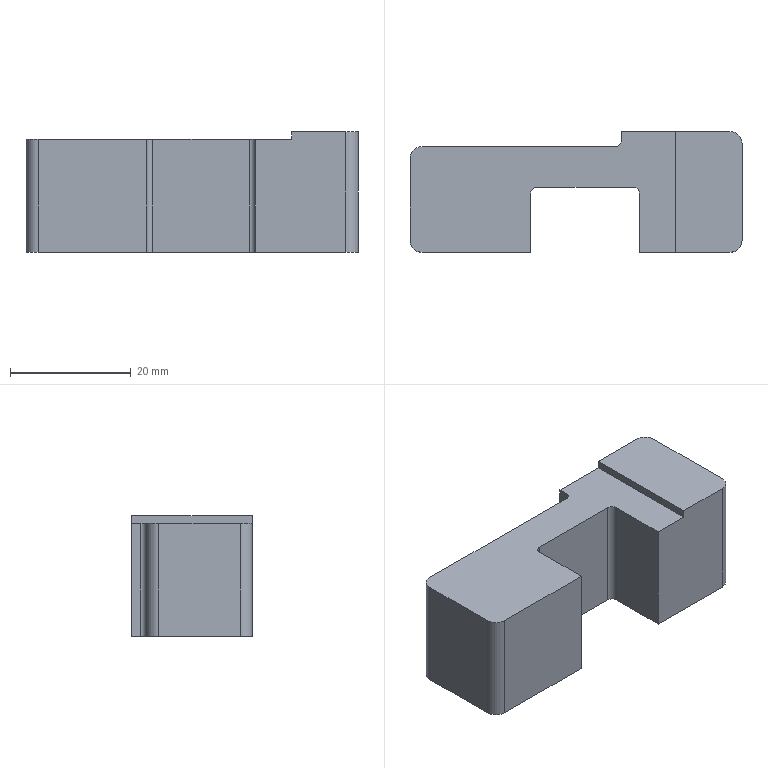Part | STEP file | 03-20 product pre-press block | 1 solid | 29 faces | box 55 x 20 x 20 mm | volume 15350 mm3 | plane 14 | cylinder 11 | cone 4 | commonest cylinder face diameters 3.3 x4 4 x4 2 x3
STEP:
#1=CARTESIAN_POINT('',(21.15,0.,10.1));
#2=VERTEX_POINT('',#1);
#3=CARTESIAN_POINT('',(17.85,0.,10.1));
#4=VERTEX_POINT('',#3);
#5=CARTESIAN_POINT('',(19.5,0.,10.1));
#6=DIRECTION('',(0.,0.,-1.));
#7=DIRECTION('',(-1.,0.,0.));
#8=AXIS2_PLACEMENT_3D('',#5,#6,#7);
#9=CIRCLE('',#8,1.65);
#10=EDGE_CURVE('',#2,#4,#9,.T.);
#11=ORIENTED_EDGE('',*,*,#10,.F.);
#12=CARTESIAN_POINT('',(21.15,0.,0.));
#13=VERTEX_POINT('',#12);
#14=CARTESIAN_POINT('',(21.15,0.,0.));
#15=DIRECTION('',(0.,0.,-1.));
#16=VECTOR('',#15,1000.);
#17=LINE('',#14,#16);
#18=EDGE_CURVE('',#2,#13,#17,.T.);
#19=ORIENTED_EDGE('',*,*,#18,.T.);
#20=CARTESIAN_POINT('',(17.85,0.,0.));
#21=VERTEX_POINT('',#20);
#22=CARTESIAN_POINT('',(19.5,0.,0.));
#23=DIRECTION('',(0.,0.,-1.));
#24=DIRECTION('',(-1.,0.,0.));
#25=AXIS2_PLACEMENT_3D('',#22,#23,#24);
#26=CIRCLE('',#25,1.65);
#27=EDGE_CURVE('',#13,#21,#26,.T.);
#28=ORIENTED_EDGE('',*,*,#27,.T.);
#29=CARTESIAN_POINT('',(17.85,0.,0.));
#30=DIRECTION('',(0.,0.,-1.));
#31=VECTOR('',#30,1000.);
#32=LINE('',#29,#31);
#33=EDGE_CURVE('',#4,#21,#32,.T.);
#34=ORIENTED_EDGE('',*,*,#33,.F.);
#35=EDGE_LOOP('',(#11,#19,#28,#34));
#36=FACE_OUTER_BOUND('',#35,.T.);
#37=CARTESIAN_POINT('',(19.5,0.,0.));
#38=DIRECTION('',(0.,0.,-1.));
#39=DIRECTION('',(-1.,0.,0.));
#40=AXIS2_PLACEMENT_3D('',#37,#38,#39);
#41=CYLINDRICAL_SURFACE('',#40,1.65);
#42=ADVANCED_FACE('',(#36),#41,.F.);
#43=CARTESIAN_POINT('',(19.5,0.,11.091));
#44=VERTEX_POINT('',#43);
#45=CARTESIAN_POINT('',(17.85,0.,10.1));
#46=DIRECTION('',(-0.8572,0.,-0.515));
#47=VECTOR('',#46,1000.);
#48=LINE('',#45,#47);
#49=EDGE_CURVE('',#44,#4,#48,.T.);
#50=ORIENTED_EDGE('',*,*,#49,.F.);
#51=CARTESIAN_POINT('',(21.15,0.,10.1));
#52=DIRECTION('',(0.8572,0.,-0.515));
#53=VECTOR('',#52,1000.);
#54=LINE('',#51,#53);
#55=EDGE_CURVE('',#44,#2,#54,.T.);
#56=ORIENTED_EDGE('',*,*,#55,.T.);
#57=ORIENTED_EDGE('',*,*,#10,.T.);
#58=EDGE_LOOP('',(#50,#56,#57));
#59=FACE_OUTER_BOUND('',#58,.T.);
#60=CARTESIAN_POINT('',(19.5,0.,10.1));
#61=DIRECTION('',(0.,0.,-1.));
#62=DIRECTION('',(-1.,0.,0.));
#63=AXIS2_PLACEMENT_3D('',#60,#61,#62);
#64=CONICAL_SURFACE('',#63,1.65,1.03);
#65=ADVANCED_FACE('',(#59),#64,.F.);
#66=CARTESIAN_POINT('',(-17.85,0.,10.1));
#67=VERTEX_POINT('',#66);
#68=CARTESIAN_POINT('',(-21.15,0.,10.1));
#69=VERTEX_POINT('',#68);
#70=CARTESIAN_POINT('',(-19.5,0.,10.1));
#71=DIRECTION('',(0.,0.,-1.));
#72=DIRECTION('',(-1.,0.,0.));
#73=AXIS2_PLACEMENT_3D('',#70,#71,#72);
#74=CIRCLE('',#73,1.65);
#75=EDGE_CURVE('',#67,#69,#74,.T.);
#76=ORIENTED_EDGE('',*,*,#75,.F.);
#77=CARTESIAN_POINT('',(-17.85,0.,0.));
#78=VERTEX_POINT('',#77);
#79=CARTESIAN_POINT('',(-17.85,0.,0.));
#80=DIRECTION('',(0.,0.,-1.));
#81=VECTOR('',#80,1000.);
#82=LINE('',#79,#81);
#83=EDGE_CURVE('',#67,#78,#82,.T.);
#84=ORIENTED_EDGE('',*,*,#83,.T.);
#85=CARTESIAN_POINT('',(-21.15,0.,0.));
#86=VERTEX_POINT('',#85);
#87=CARTESIAN_POINT('',(-19.5,0.,0.));
#88=DIRECTION('',(0.,0.,-1.));
#89=DIRECTION('',(-1.,0.,0.));
#90=AXIS2_PLACEMENT_3D('',#87,#88,#89);
#91=CIRCLE('',#90,1.65);
#92=EDGE_CURVE('',#78,#86,#91,.T.);
#93=ORIENTED_EDGE('',*,*,#92,.T.);
#94=CARTESIAN_POINT('',(-21.15,0.,0.));
#95=DIRECTION('',(0.,0.,-1.));
#96=VECTOR('',#95,1000.);
#97=LINE('',#94,#96);
#98=EDGE_CURVE('',#69,#86,#97,.T.);
#99=ORIENTED_EDGE('',*,*,#98,.F.);
#100=EDGE_LOOP('',(#76,#84,#93,#99));
#101=FACE_OUTER_BOUND('',#100,.T.);
#102=CARTESIAN_POINT('',(-19.5,0.,0.));
#103=DIRECTION('',(0.,0.,-1.));
#104=DIRECTION('',(-1.,0.,0.));
#105=AXIS2_PLACEMENT_3D('',#102,#103,#104);
#106=CYLINDRICAL_SURFACE('',#105,1.65);
#107=ADVANCED_FACE('',(#101),#106,.F.);
#108=CARTESIAN_POINT('',(-19.5,0.,11.091));
#109=VERTEX_POINT('',#108);
#110=CARTESIAN_POINT('',(-21.15,0.,10.1));
#111=DIRECTION('',(-0.8572,0.,-0.515));
#112=VECTOR('',#111,1000.);
#113=LINE('',#110,#112);
#114=EDGE_CURVE('',#109,#69,#113,.T.);
#115=ORIENTED_EDGE('',*,*,#114,.F.);
#116=CARTESIAN_POINT('',(-17.85,0.,10.1));
#117=DIRECTION('',(0.8572,0.,-0.515));
#118=VECTOR('',#117,1000.);
#119=LINE('',#116,#118);
#120=EDGE_CURVE('',#109,#67,#119,.T.);
#121=ORIENTED_EDGE('',*,*,#120,.T.);
#122=ORIENTED_EDGE('',*,*,#75,.T.);
#123=EDGE_LOOP('',(#115,#121,#122));
#124=FACE_OUTER_BOUND('',#123,.T.);
#125=CARTESIAN_POINT('',(-19.5,0.,10.1));
#126=DIRECTION('',(0.,0.,-1.));
#127=DIRECTION('',(-1.,0.,0.));
#128=AXIS2_PLACEMENT_3D('',#125,#126,#127);
#129=CONICAL_SURFACE('',#128,1.65,1.03);
#130=ADVANCED_FACE('',(#124),#129,.F.);
#131=CARTESIAN_POINT('',(19.5,0.,0.));
#132=DIRECTION('',(0.,0.,-1.));
#133=DIRECTION('',(-1.,0.,0.));
#134=AXIS2_PLACEMENT_3D('',#131,#132,#133);
#135=CIRCLE('',#134,1.65);
#136=EDGE_CURVE('',#21,#13,#135,.T.);
#137=ORIENTED_EDGE('',*,*,#136,.F.);
#138=ORIENTED_EDGE('',*,*,#27,.F.);
#139=EDGE_LOOP('',(#137,#138));
#140=FACE_BOUND('',#139,.T.);
#141=CARTESIAN_POINT('',(25.5,10.,0.));
#142=VERTEX_POINT('',#141);
#143=CARTESIAN_POINT('',(7.5,10.,0.));
#144=VERTEX_POINT('',#143);
#145=CARTESIAN_POINT('',(-27.5,10.,0.));
#146=DIRECTION('',(-1.,0.,0.));
#147=VECTOR('',#146,1000.);
#148=LINE('',#145,#147);
#149=EDGE_CURVE('',#142,#144,#148,.T.);
#150=ORIENTED_EDGE('',*,*,#149,.F.);
#151=CARTESIAN_POINT('',(27.5,8.,0.));
#152=VERTEX_POINT('',#151);
#153=CARTESIAN_POINT('',(25.5,8.,0.));
#154=DIRECTION('',(0.,0.,-1.));
#155=DIRECTION('',(1.,0.,0.));
#156=AXIS2_PLACEMENT_3D('',#153,#154,#155);
#157=CIRCLE('',#156,2.);
#158=EDGE_CURVE('',#142,#152,#157,.T.);
#159=ORIENTED_EDGE('',*,*,#158,.T.);
#160=CARTESIAN_POINT('',(27.5,-8.,0.));
#161=VERTEX_POINT('',#160);
#162=CARTESIAN_POINT('',(27.5,10.,0.));
#163=DIRECTION('',(0.,1.,0.));
#164=VECTOR('',#163,1000.);
#165=LINE('',#162,#164);
#166=EDGE_CURVE('',#161,#152,#165,.T.);
#167=ORIENTED_EDGE('',*,*,#166,.F.);
#168=CARTESIAN_POINT('',(25.5,-10.,0.));
#169=VERTEX_POINT('',#168);
#170=CARTESIAN_POINT('',(25.5,-8.,0.));
#171=DIRECTION('',(0.,0.,-1.));
#172=DIRECTION('',(1.,0.,0.));
#173=AXIS2_PLACEMENT_3D('',#170,#171,#172);
#174=CIRCLE('',#173,2.);
#175=EDGE_CURVE('',#161,#169,#174,.T.);
#176=ORIENTED_EDGE('',*,*,#175,.T.);
#177=CARTESIAN_POINT('',(10.5,-10.,0.));
#178=VERTEX_POINT('',#177);
#179=CARTESIAN_POINT('',(-27.5,-10.,0.));
#180=DIRECTION('',(1.,0.,0.));
#181=VECTOR('',#180,1000.);
#182=LINE('',#179,#181);
#183=EDGE_CURVE('',#178,#169,#182,.T.);
#184=ORIENTED_EDGE('',*,*,#183,.F.);
#185=CARTESIAN_POINT('',(10.5,-0.1961,0.));
#186=VERTEX_POINT('',#185);
#187=CARTESIAN_POINT('',(10.5,-10.,0.));
#188=DIRECTION('',(0.,-1.,0.));
#189=VECTOR('',#188,1000.);
#190=LINE('',#187,#189);
#191=EDGE_CURVE('',#186,#178,#190,.T.);
#192=ORIENTED_EDGE('',*,*,#191,.F.);
#193=CARTESIAN_POINT('',(9.5,0.8039,0.));
#194=VERTEX_POINT('',#193);
#195=CARTESIAN_POINT('',(9.5,-0.1961,0.));
#196=DIRECTION('',(0.,0.,1.));
#197=DIRECTION('',(1.,0.,0.));
#198=AXIS2_PLACEMENT_3D('',#195,#196,#197);
#199=CIRCLE('',#198,1.);
#200=EDGE_CURVE('',#186,#194,#199,.T.);
#201=ORIENTED_EDGE('',*,*,#200,.T.);
#202=CARTESIAN_POINT('',(-6.5,0.8039,0.));
#203=VERTEX_POINT('',#202);
#204=CARTESIAN_POINT('',(10.5,0.8039,0.));
#205=DIRECTION('',(1.,0.,0.));
#206=VECTOR('',#205,1000.);
#207=LINE('',#204,#206);
#208=EDGE_CURVE('',#203,#194,#207,.T.);
#209=ORIENTED_EDGE('',*,*,#208,.F.);
#210=CARTESIAN_POINT('',(-7.5,-0.1961,0.));
#211=VERTEX_POINT('',#210);
#212=CARTESIAN_POINT('',(-6.5,-0.1961,0.));
#213=DIRECTION('',(0.,0.,1.));
#214=DIRECTION('',(1.,0.,0.));
#215=AXIS2_PLACEMENT_3D('',#212,#213,#214);
#216=CIRCLE('',#215,1.);
#217=EDGE_CURVE('',#203,#211,#216,.T.);
#218=ORIENTED_EDGE('',*,*,#217,.T.);
#219=CARTESIAN_POINT('',(-7.5,-10.,0.));
#220=VERTEX_POINT('',#219);
#221=CARTESIAN_POINT('',(-7.5,-10.,0.));
#222=DIRECTION('',(0.,1.,0.));
#223=VECTOR('',#222,1000.);
#224=LINE('',#221,#223);
#225=EDGE_CURVE('',#220,#211,#224,.T.);
#226=ORIENTED_EDGE('',*,*,#225,.F.);
#227=CARTESIAN_POINT('',(-25.5,-10.,0.));
#228=VERTEX_POINT('',#227);
#229=CARTESIAN_POINT('',(-27.5,-10.,0.));
#230=DIRECTION('',(1.,0.,0.));
#231=VECTOR('',#230,1000.);
#232=LINE('',#229,#231);
#233=EDGE_CURVE('',#228,#220,#232,.T.);
#234=ORIENTED_EDGE('',*,*,#233,.F.);
#235=CARTESIAN_POINT('',(-27.5,-8.,0.));
#236=VERTEX_POINT('',#235);
#237=CARTESIAN_POINT('',(-25.5,-8.,0.));
#238=DIRECTION('',(0.,0.,-1.));
#239=DIRECTION('',(1.,0.,0.));
#240=AXIS2_PLACEMENT_3D('',#237,#238,#239);
#241=CIRCLE('',#240,2.);
#242=EDGE_CURVE('',#228,#236,#241,.T.);
#243=ORIENTED_EDGE('',*,*,#242,.T.);
#244=CARTESIAN_POINT('',(-27.5,5.5,0.));
#245=VERTEX_POINT('',#244);
#246=CARTESIAN_POINT('',(-27.5,10.,0.));
#247=DIRECTION('',(0.,-1.,0.));
#248=VECTOR('',#247,1000.);
#249=LINE('',#246,#248);
#250=EDGE_CURVE('',#245,#236,#249,.T.);
#251=ORIENTED_EDGE('',*,*,#250,.F.);
#252=CARTESIAN_POINT('',(-25.5,7.5,0.));
#253=VERTEX_POINT('',#252);
#254=CARTESIAN_POINT('',(-25.5,5.5,0.));
#255=DIRECTION('',(0.,0.,-1.));
#256=DIRECTION('',(1.,0.,0.));
#257=AXIS2_PLACEMENT_3D('',#254,#255,#256);
#258=CIRCLE('',#257,2.);
#259=EDGE_CURVE('',#245,#253,#258,.T.);
#260=ORIENTED_EDGE('',*,*,#259,.T.);
#261=CARTESIAN_POINT('',(6.5,7.5,0.));
#262=VERTEX_POINT('',#261);
#263=CARTESIAN_POINT('',(7.5,7.5,0.));
#264=DIRECTION('',(-1.,0.,0.));
#265=VECTOR('',#264,1000.);
#266=LINE('',#263,#265);
#267=EDGE_CURVE('',#262,#253,#266,.T.);
#268=ORIENTED_EDGE('',*,*,#267,.F.);
#269=CARTESIAN_POINT('',(7.5,8.5,0.));
#270=VERTEX_POINT('',#269);
#271=CARTESIAN_POINT('',(6.5,8.5,0.));
#272=DIRECTION('',(0.,0.,1.));
#273=DIRECTION('',(1.,0.,0.));
#274=AXIS2_PLACEMENT_3D('',#271,#272,#273);
#275=CIRCLE('',#274,1.);
#276=EDGE_CURVE('',#262,#270,#275,.T.);
#277=ORIENTED_EDGE('',*,*,#276,.T.);
#278=CARTESIAN_POINT('',(7.5,10.,0.));
#279=DIRECTION('',(0.,-1.,0.));
#280=VECTOR('',#279,1000.);
#281=LINE('',#278,#280);
#282=EDGE_CURVE('',#144,#270,#281,.T.);
#283=ORIENTED_EDGE('',*,*,#282,.F.);
#284=EDGE_LOOP('',(#150,#159,#167,#176,#184,#192,#201,#209,#218,#226,#234,#243,#251,#260,#268,#277,#283));
#285=FACE_OUTER_BOUND('',#284,.T.);
#286=CARTESIAN_POINT('',(-19.5,0.,0.));
#287=DIRECTION('',(0.,0.,-1.));
#288=DIRECTION('',(-1.,0.,0.));
#289=AXIS2_PLACEMENT_3D('',#286,#287,#288);
#290=CIRCLE('',#289,1.65);
#291=EDGE_CURVE('',#86,#78,#290,.T.);
#292=ORIENTED_EDGE('',*,*,#291,.F.);
#293=ORIENTED_EDGE('',*,*,#92,.F.);
#294=EDGE_LOOP('',(#292,#293));
#295=FACE_BOUND('',#294,.T.);
#296=CARTESIAN_POINT('',(27.5,-10.,0.));
#297=DIRECTION('',(0.,0.,1.));
#298=DIRECTION('',(1.,0.,0.));
#299=AXIS2_PLACEMENT_3D('',#296,#297,#298);
#300=PLANE('',#299);
#301=ADVANCED_FACE('',(#140,#285,#295),#300,.F.);
#302=ORIENTED_EDGE('',*,*,#183,.T.);
#303=CARTESIAN_POINT('',(25.5,-10.,20.));
#304=VERTEX_POINT('',#303);
#305=CARTESIAN_POINT('',(25.5,-10.,20.));
#306=DIRECTION('',(0.,0.,1.));
#307=VECTOR('',#306,1000.);
#308=LINE('',#305,#307);
#309=EDGE_CURVE('',#169,#304,#308,.T.);
#310=ORIENTED_EDGE('',*,*,#309,.T.);
#311=CARTESIAN_POINT('',(16.5,-10.,20.));
#312=VERTEX_POINT('',#311);
#313=CARTESIAN_POINT('',(-27.5,-10.,20.));
#314=DIRECTION('',(1.,0.,0.));
#315=VECTOR('',#314,1000.);
#316=LINE('',#313,#315);
#317=EDGE_CURVE('',#312,#304,#316,.T.);
#318=ORIENTED_EDGE('',*,*,#317,.F.);
#319=CARTESIAN_POINT('',(16.5,-10.,18.7));
#320=VERTEX_POINT('',#319);
#321=CARTESIAN_POINT('',(16.5,-10.,20.));
#322=DIRECTION('',(0.,0.,1.));
#323=VECTOR('',#322,1000.);
#324=LINE('',#321,#323);
#325=EDGE_CURVE('',#320,#312,#324,.T.);
#326=ORIENTED_EDGE('',*,*,#325,.F.);
#327=CARTESIAN_POINT('',(10.5,-10.,18.7));
#328=VERTEX_POINT('',#327);
#329=CARTESIAN_POINT('',(-27.5,-10.,18.7));
#330=DIRECTION('',(1.,0.,0.));
#331=VECTOR('',#330,1000.);
#332=LINE('',#329,#331);
#333=EDGE_CURVE('',#328,#320,#332,.T.);
#334=ORIENTED_EDGE('',*,*,#333,.F.);
#335=CARTESIAN_POINT('',(10.5,-10.,20.));
#336=DIRECTION('',(0.,0.,-1.));
#337=VECTOR('',#336,1000.);
#338=LINE('',#335,#337);
#339=EDGE_CURVE('',#328,#178,#338,.T.);
#340=ORIENTED_EDGE('',*,*,#339,.T.);
#341=EDGE_LOOP('',(#302,#310,#318,#326,#334,#340));
#342=FACE_OUTER_BOUND('',#341,.T.);
#343=CARTESIAN_POINT('',(-27.5,-10.,20.));
#344=DIRECTION('',(0.,1.,0.));
#345=DIRECTION('',(0.,0.,1.));
#346=AXIS2_PLACEMENT_3D('',#343,#344,#345);
#347=PLANE('',#346);
#348=ADVANCED_FACE('',(#342),#347,.F.);
#349=ORIENTED_EDGE('',*,*,#166,.T.);
#350=CARTESIAN_POINT('',(27.5,8.,20.));
#351=VERTEX_POINT('',#350);
#352=CARTESIAN_POINT('',(27.5,8.,20.));
#353=DIRECTION('',(0.,0.,1.));
#354=VECTOR('',#353,1000.);
#355=LINE('',#352,#354);
#356=EDGE_CURVE('',#152,#351,#355,.T.);
#357=ORIENTED_EDGE('',*,*,#356,.T.);
#358=CARTESIAN_POINT('',(27.5,-8.,20.));
#359=VERTEX_POINT('',#358);
#360=CARTESIAN_POINT('',(27.5,10.,20.));
#361=DIRECTION('',(0.,1.,0.));
#362=VECTOR('',#361,1000.);
#363=LINE('',#360,#362);
#364=EDGE_CURVE('',#359,#351,#363,.T.);
#365=ORIENTED_EDGE('',*,*,#364,.F.);
#366=CARTESIAN_POINT('',(27.5,-8.,20.));
#367=DIRECTION('',(0.,0.,-1.));
#368=VECTOR('',#367,1000.);
#369=LINE('',#366,#368);
#370=EDGE_CURVE('',#359,#161,#369,.T.);
#371=ORIENTED_EDGE('',*,*,#370,.T.);
#372=EDGE_LOOP('',(#349,#357,#365,#371));
#373=FACE_OUTER_BOUND('',#372,.T.);
#374=CARTESIAN_POINT('',(27.5,10.,20.));
#375=DIRECTION('',(-1.,0.,0.));
#376=DIRECTION('',(0.,-1.,0.));
#377=AXIS2_PLACEMENT_3D('',#374,#375,#376);
#378=PLANE('',#377);
#379=ADVANCED_FACE('',(#373),#378,.F.);
#380=CARTESIAN_POINT('',(25.5,10.,20.));
#381=VERTEX_POINT('',#380);
#382=CARTESIAN_POINT('',(16.5,10.,20.));
#383=VERTEX_POINT('',#382);
#384=CARTESIAN_POINT('',(-27.5,10.,20.));
#385=DIRECTION('',(-1.,0.,0.));
#386=VECTOR('',#385,1000.);
#387=LINE('',#384,#386);
#388=EDGE_CURVE('',#381,#383,#387,.T.);
#389=ORIENTED_EDGE('',*,*,#388,.F.);
#390=CARTESIAN_POINT('',(25.5,10.,20.));
#391=DIRECTION('',(0.,0.,-1.));
#392=VECTOR('',#391,1000.);
#393=LINE('',#390,#392);
#394=EDGE_CURVE('',#381,#142,#393,.T.);
#395=ORIENTED_EDGE('',*,*,#394,.T.);
#396=ORIENTED_EDGE('',*,*,#149,.T.);
#397=CARTESIAN_POINT('',(7.5,10.,18.7));
#398=VERTEX_POINT('',#397);
#399=CARTESIAN_POINT('',(7.5,10.,20.));
#400=DIRECTION('',(0.,0.,-1.));
#401=VECTOR('',#400,1000.);
#402=LINE('',#399,#401);
#403=EDGE_CURVE('',#398,#144,#402,.T.);
#404=ORIENTED_EDGE('',*,*,#403,.F.);
#405=CARTESIAN_POINT('',(16.5,10.,18.7));
#406=VERTEX_POINT('',#405);
#407=CARTESIAN_POINT('',(-27.5,10.,18.7));
#408=DIRECTION('',(1.,0.,0.));
#409=VECTOR('',#408,1000.);
#410=LINE('',#407,#409);
#411=EDGE_CURVE('',#398,#406,#410,.T.);
#412=ORIENTED_EDGE('',*,*,#411,.T.);
#413=CARTESIAN_POINT('',(16.5,10.,20.));
#414=DIRECTION('',(0.,0.,1.));
#415=VECTOR('',#414,1000.);
#416=LINE('',#413,#415);
#417=EDGE_CURVE('',#406,#383,#416,.T.);
#418=ORIENTED_EDGE('',*,*,#417,.T.);
#419=EDGE_LOOP('',(#389,#395,#396,#404,#412,#418));
#420=FACE_OUTER_BOUND('',#419,.T.);
#421=CARTESIAN_POINT('',(-27.5,10.,20.));
#422=DIRECTION('',(0.,-1.,0.));
#423=DIRECTION('',(0.,0.,-1.));
#424=AXIS2_PLACEMENT_3D('',#421,#422,#423);
#425=PLANE('',#424);
#426=ADVANCED_FACE('',(#420),#425,.F.);
#427=CARTESIAN_POINT('',(-27.5,5.5,18.7));
#428=VERTEX_POINT('',#427);
#429=CARTESIAN_POINT('',(-27.5,-8.,18.7));
#430=VERTEX_POINT('',#429);
#431=CARTESIAN_POINT('',(-27.5,10.,18.7));
#432=DIRECTION('',(0.,-1.,0.));
#433=VECTOR('',#432,1000.);
#434=LINE('',#431,#433);
#435=EDGE_CURVE('',#428,#430,#434,.T.);
#436=ORIENTED_EDGE('',*,*,#435,.F.);
#437=CARTESIAN_POINT('',(-27.5,5.5,20.));
#438=DIRECTION('',(0.,0.,-1.));
#439=VECTOR('',#438,1000.);
#440=LINE('',#437,#439);
#441=EDGE_CURVE('',#428,#245,#440,.T.);
#442=ORIENTED_EDGE('',*,*,#441,.T.);
#443=ORIENTED_EDGE('',*,*,#250,.T.);
#444=CARTESIAN_POINT('',(-27.5,-8.,20.));
#445=DIRECTION('',(0.,0.,1.));
#446=VECTOR('',#445,1000.);
#447=LINE('',#444,#446);
#448=EDGE_CURVE('',#236,#430,#447,.T.);
#449=ORIENTED_EDGE('',*,*,#448,.T.);
#450=EDGE_LOOP('',(#436,#442,#443,#449));
#451=FACE_OUTER_BOUND('',#450,.T.);
#452=CARTESIAN_POINT('',(-27.5,10.,20.));
#453=DIRECTION('',(1.,0.,0.));
#454=DIRECTION('',(0.,1.,0.));
#455=AXIS2_PLACEMENT_3D('',#452,#453,#454);
#456=PLANE('',#455);
#457=ADVANCED_FACE('',(#451),#456,.F.);
#458=CARTESIAN_POINT('',(-25.5,-10.,18.7));
#459=VERTEX_POINT('',#458);
#460=CARTESIAN_POINT('',(-7.5,-10.,18.7));
#461=VERTEX_POINT('',#460);
#462=CARTESIAN_POINT('',(-27.5,-10.,18.7));
#463=DIRECTION('',(1.,0.,0.));
#464=VECTOR('',#463,1000.);
#465=LINE('',#462,#464);
#466=EDGE_CURVE('',#459,#461,#465,.T.);
#467=ORIENTED_EDGE('',*,*,#466,.F.);
#468=CARTESIAN_POINT('',(-25.5,-10.,20.));
#469=DIRECTION('',(0.,0.,-1.));
#470=VECTOR('',#469,1000.);
#471=LINE('',#468,#470);
#472=EDGE_CURVE('',#459,#228,#471,.T.);
#473=ORIENTED_EDGE('',*,*,#472,.T.);
#474=ORIENTED_EDGE('',*,*,#233,.T.);
#475=CARTESIAN_POINT('',(-7.5,-10.,20.));
#476=DIRECTION('',(0.,0.,-1.));
#477=VECTOR('',#476,1000.);
#478=LINE('',#475,#477);
#479=EDGE_CURVE('',#461,#220,#478,.T.);
#480=ORIENTED_EDGE('',*,*,#479,.F.);
#481=EDGE_LOOP('',(#467,#473,#474,#480));
#482=FACE_OUTER_BOUND('',#481,.T.);
#483=CARTESIAN_POINT('',(-27.5,-10.,20.));
#484=DIRECTION('',(0.,1.,0.));
#485=DIRECTION('',(0.,0.,1.));
#486=AXIS2_PLACEMENT_3D('',#483,#484,#485);
#487=PLANE('',#486);
#488=ADVANCED_FACE('',(#482),#487,.F.);
#489=ORIENTED_EDGE('',*,*,#364,.T.);
#490=CARTESIAN_POINT('',(25.5,8.,20.));
#491=DIRECTION('',(0.,0.,1.));
#492=DIRECTION('',(1.,0.,0.));
#493=AXIS2_PLACEMENT_3D('',#490,#491,#492);
#494=CIRCLE('',#493,2.);
#495=EDGE_CURVE('',#351,#381,#494,.T.);
#496=ORIENTED_EDGE('',*,*,#495,.T.);
#497=ORIENTED_EDGE('',*,*,#388,.T.);
#498=CARTESIAN_POINT('',(16.5,10.,20.));
#499=DIRECTION('',(0.,-1.,0.));
#500=VECTOR('',#499,1000.);
#501=LINE('',#498,#500);
#502=EDGE_CURVE('',#383,#312,#501,.T.);
#503=ORIENTED_EDGE('',*,*,#502,.T.);
#504=ORIENTED_EDGE('',*,*,#317,.T.);
#505=CARTESIAN_POINT('',(25.5,-8.,20.));
#506=DIRECTION('',(0.,0.,1.));
#507=DIRECTION('',(1.,0.,0.));
#508=AXIS2_PLACEMENT_3D('',#505,#506,#507);
#509=CIRCLE('',#508,2.);
#510=EDGE_CURVE('',#304,#359,#509,.T.);
#511=ORIENTED_EDGE('',*,*,#510,.T.);
#512=EDGE_LOOP('',(#489,#496,#497,#503,#504,#511));
#513=FACE_OUTER_BOUND('',#512,.T.);
#514=CARTESIAN_POINT('',(27.5,-10.,20.));
#515=DIRECTION('',(0.,0.,1.));
#516=DIRECTION('',(1.,0.,0.));
#517=AXIS2_PLACEMENT_3D('',#514,#515,#516);
#518=PLANE('',#517);
#519=ADVANCED_FACE('',(#513),#518,.T.);
#520=ORIENTED_EDGE('',*,*,#325,.T.);
#521=ORIENTED_EDGE('',*,*,#502,.F.);
#522=ORIENTED_EDGE('',*,*,#417,.F.);
#523=CARTESIAN_POINT('',(16.5,10.,18.7));
#524=DIRECTION('',(0.,-1.,0.));
#525=VECTOR('',#524,1000.);
#526=LINE('',#523,#525);
#527=EDGE_CURVE('',#406,#320,#526,.T.);
#528=ORIENTED_EDGE('',*,*,#527,.T.);
#529=EDGE_LOOP('',(#520,#521,#522,#528));
#530=FACE_OUTER_BOUND('',#529,.T.);
#531=CARTESIAN_POINT('',(16.5,10.,20.));
#532=DIRECTION('',(1.,0.,0.));
#533=DIRECTION('',(0.,0.,-1.));
#534=AXIS2_PLACEMENT_3D('',#531,#532,#533);
#535=PLANE('',#534);
#536=ADVANCED_FACE('',(#530),#535,.F.);
#537=CARTESIAN_POINT('',(6.5,7.5,18.7));
#538=VERTEX_POINT('',#537);
#539=CARTESIAN_POINT('',(-25.5,7.5,18.7));
#540=VERTEX_POINT('',#539);
#541=CARTESIAN_POINT('',(-27.5,7.5,18.7));
#542=DIRECTION('',(-1.,0.,0.));
#543=VECTOR('',#542,1000.);
#544=LINE('',#541,#543);
#545=EDGE_CURVE('',#538,#540,#544,.T.);
#546=ORIENTED_EDGE('',*,*,#545,.T.);
#547=CARTESIAN_POINT('',(-25.5,5.5,18.7));
#548=DIRECTION('',(0.,0.,1.));
#549=DIRECTION('',(-1.,0.,0.));
#550=AXIS2_PLACEMENT_3D('',#547,#548,#549);
#551=CIRCLE('',#550,2.);
#552=EDGE_CURVE('',#540,#428,#551,.T.);
#553=ORIENTED_EDGE('',*,*,#552,.T.);
#554=ORIENTED_EDGE('',*,*,#435,.T.);
#555=CARTESIAN_POINT('',(-25.5,-8.,18.7));
#556=DIRECTION('',(0.,0.,1.));
#557=DIRECTION('',(-1.,0.,0.));
#558=AXIS2_PLACEMENT_3D('',#555,#556,#557);
#559=CIRCLE('',#558,2.);
#560=EDGE_CURVE('',#430,#459,#559,.T.);
#561=ORIENTED_EDGE('',*,*,#560,.T.);
#562=ORIENTED_EDGE('',*,*,#466,.T.);
#563=CARTESIAN_POINT('',(-7.5,-0.1961,18.7));
#564=VERTEX_POINT('',#563);
#565=CARTESIAN_POINT('',(-7.5,10.,18.7));
#566=DIRECTION('',(0.,1.,0.));
#567=VECTOR('',#566,1000.);
#568=LINE('',#565,#567);
#569=EDGE_CURVE('',#461,#564,#568,.T.);
#570=ORIENTED_EDGE('',*,*,#569,.T.);
#571=CARTESIAN_POINT('',(-6.5,0.8039,18.7));
#572=VERTEX_POINT('',#571);
#573=CARTESIAN_POINT('',(-6.5,-0.1961,18.7));
#574=DIRECTION('',(0.,0.,-1.));
#575=DIRECTION('',(-1.,0.,0.));
#576=AXIS2_PLACEMENT_3D('',#573,#574,#575);
#577=CIRCLE('',#576,1.);
#578=EDGE_CURVE('',#564,#572,#577,.T.);
#579=ORIENTED_EDGE('',*,*,#578,.T.);
#580=CARTESIAN_POINT('',(9.5,0.8039,18.7));
#581=VERTEX_POINT('',#580);
#582=CARTESIAN_POINT('',(-27.5,0.8039,18.7));
#583=DIRECTION('',(1.,0.,0.));
#584=VECTOR('',#583,1000.);
#585=LINE('',#582,#584);
#586=EDGE_CURVE('',#572,#581,#585,.T.);
#587=ORIENTED_EDGE('',*,*,#586,.T.);
#588=CARTESIAN_POINT('',(10.5,-0.1961,18.7));
#589=VERTEX_POINT('',#588);
#590=CARTESIAN_POINT('',(9.5,-0.1961,18.7));
#591=DIRECTION('',(0.,0.,-1.));
#592=DIRECTION('',(-1.,0.,0.));
#593=AXIS2_PLACEMENT_3D('',#590,#591,#592);
#594=CIRCLE('',#593,1.);
#595=EDGE_CURVE('',#581,#589,#594,.T.);
#596=ORIENTED_EDGE('',*,*,#595,.T.);
#597=CARTESIAN_POINT('',(10.5,10.,18.7));
#598=DIRECTION('',(0.,-1.,0.));
#599=VECTOR('',#598,1000.);
#600=LINE('',#597,#599);
#601=EDGE_CURVE('',#589,#328,#600,.T.);
#602=ORIENTED_EDGE('',*,*,#601,.T.);
#603=ORIENTED_EDGE('',*,*,#333,.T.);
#604=ORIENTED_EDGE('',*,*,#527,.F.);
#605=ORIENTED_EDGE('',*,*,#411,.F.);
#606=CARTESIAN_POINT('',(7.5,8.5,18.7));
#607=VERTEX_POINT('',#606);
#608=CARTESIAN_POINT('',(7.5,10.,18.7));
#609=DIRECTION('',(0.,-1.,0.));
#610=VECTOR('',#609,1000.);
#611=LINE('',#608,#610);
#612=EDGE_CURVE('',#398,#607,#611,.T.);
#613=ORIENTED_EDGE('',*,*,#612,.T.);
#614=CARTESIAN_POINT('',(6.5,8.5,18.7));
#615=DIRECTION('',(0.,0.,-1.));
#616=DIRECTION('',(-1.,0.,0.));
#617=AXIS2_PLACEMENT_3D('',#614,#615,#616);
#618=CIRCLE('',#617,1.);
#619=EDGE_CURVE('',#607,#538,#618,.T.);
#620=ORIENTED_EDGE('',*,*,#619,.T.);
#621=EDGE_LOOP('',(#546,#553,#554,#561,#562,#570,#579,#587,#596,#602,#603,#604,#605,#613,#620));
#622=FACE_OUTER_BOUND('',#621,.T.);
#623=CARTESIAN_POINT('',(-27.5,10.,18.7));
#624=DIRECTION('',(0.,0.,-1.));
#625=DIRECTION('',(-1.,0.,0.));
#626=AXIS2_PLACEMENT_3D('',#623,#624,#625);
#627=PLANE('',#626);
#628=ADVANCED_FACE('',(#622),#627,.F.);
#629=ORIENTED_EDGE('',*,*,#282,.T.);
#630=CARTESIAN_POINT('',(7.5,8.5,18.7));
#631=DIRECTION('',(0.,0.,1.));
#632=VECTOR('',#631,1000.);
#633=LINE('',#630,#632);
#634=EDGE_CURVE('',#270,#607,#633,.T.);
#635=ORIENTED_EDGE('',*,*,#634,.T.);
#636=ORIENTED_EDGE('',*,*,#612,.F.);
#637=ORIENTED_EDGE('',*,*,#403,.T.);
#638=EDGE_LOOP('',(#629,#635,#636,#637));
#639=FACE_OUTER_BOUND('',#638,.T.);
#640=CARTESIAN_POINT('',(7.5,10.,20.));
#641=DIRECTION('',(1.,0.,0.));
#642=DIRECTION('',(0.,0.,-1.));
#643=AXIS2_PLACEMENT_3D('',#640,#641,#642);
#644=PLANE('',#643);
#645=ADVANCED_FACE('',(#639),#644,.F.);
#646=ORIENTED_EDGE('',*,*,#267,.T.);
#647=CARTESIAN_POINT('',(-25.5,7.5,20.));
#648=DIRECTION('',(0.,0.,1.));
#649=VECTOR('',#648,1000.);
#650=LINE('',#647,#649);
#651=EDGE_CURVE('',#253,#540,#650,.T.);
#652=ORIENTED_EDGE('',*,*,#651,.T.);
#653=ORIENTED_EDGE('',*,*,#545,.F.);
#654=CARTESIAN_POINT('',(6.5,7.5,0.));
#655=DIRECTION('',(0.,0.,-1.));
#656=VECTOR('',#655,1000.);
#657=LINE('',#654,#656);
#658=EDGE_CURVE('',#538,#262,#657,.T.);
#659=ORIENTED_EDGE('',*,*,#658,.T.);
#660=EDGE_LOOP('',(#646,#652,#653,#659));
#661=FACE_OUTER_BOUND('',#660,.T.);
#662=CARTESIAN_POINT('',(7.5,7.5,20.));
#663=DIRECTION('',(0.,-1.,0.));
#664=DIRECTION('',(0.,0.,-1.));
#665=AXIS2_PLACEMENT_3D('',#662,#663,#664);
#666=PLANE('',#665);
#667=ADVANCED_FACE('',(#661),#666,.F.);
#668=ORIENTED_EDGE('',*,*,#601,.F.);
#669=CARTESIAN_POINT('',(10.5,-0.1961,0.));
#670=DIRECTION('',(0.,0.,-1.));
#671=VECTOR('',#670,1000.);
#672=LINE('',#669,#671);
#673=EDGE_CURVE('',#589,#186,#672,.T.);
#674=ORIENTED_EDGE('',*,*,#673,.T.);
#675=ORIENTED_EDGE('',*,*,#191,.T.);
#676=ORIENTED_EDGE('',*,*,#339,.F.);
#677=EDGE_LOOP('',(#668,#674,#675,#676));
#678=FACE_OUTER_BOUND('',#677,.T.);
#679=CARTESIAN_POINT('',(10.5,-10.,20.));
#680=DIRECTION('',(1.,0.,0.));
#681=DIRECTION('',(0.,1.,0.));
#682=AXIS2_PLACEMENT_3D('',#679,#680,#681);
#683=PLANE('',#682);
#684=ADVANCED_FACE('',(#678),#683,.F.);
#685=ORIENTED_EDGE('',*,*,#586,.F.);
#686=CARTESIAN_POINT('',(-6.5,0.8039,0.));
#687=DIRECTION('',(0.,0.,-1.));
#688=VECTOR('',#687,1000.);
#689=LINE('',#686,#688);
#690=EDGE_CURVE('',#572,#203,#689,.T.);
#691=ORIENTED_EDGE('',*,*,#690,.T.);
#692=ORIENTED_EDGE('',*,*,#208,.T.);
#693=CARTESIAN_POINT('',(9.5,0.8039,18.7));
#694=DIRECTION('',(0.,0.,1.));
#695=VECTOR('',#694,1000.);
#696=LINE('',#693,#695);
#697=EDGE_CURVE('',#194,#581,#696,.T.);
#698=ORIENTED_EDGE('',*,*,#697,.T.);
#699=EDGE_LOOP('',(#685,#691,#692,#698));
#700=FACE_OUTER_BOUND('',#699,.T.);
#701=CARTESIAN_POINT('',(10.5,0.8039,20.));
#702=DIRECTION('',(0.,1.,0.));
#703=DIRECTION('',(0.,0.,1.));
#704=AXIS2_PLACEMENT_3D('',#701,#702,#703);
#705=PLANE('',#704);
#706=ADVANCED_FACE('',(#700),#705,.F.);
#707=ORIENTED_EDGE('',*,*,#225,.T.);
#708=CARTESIAN_POINT('',(-7.5,-0.1961,18.7));
#709=DIRECTION('',(0.,0.,1.));
#710=VECTOR('',#709,1000.);
#711=LINE('',#708,#710);
#712=EDGE_CURVE('',#211,#564,#711,.T.);
#713=ORIENTED_EDGE('',*,*,#712,.T.);
#714=ORIENTED_EDGE('',*,*,#569,.F.);
#715=ORIENTED_EDGE('',*,*,#479,.T.);
#716=EDGE_LOOP('',(#707,#713,#714,#715));
#717=FACE_OUTER_BOUND('',#716,.T.);
#718=CARTESIAN_POINT('',(-7.5,-10.,20.));
#719=DIRECTION('',(-1.,0.,0.));
#720=DIRECTION('',(0.,0.,1.));
#721=AXIS2_PLACEMENT_3D('',#718,#719,#720);
#722=PLANE('',#721);
#723=ADVANCED_FACE('',(#717),#722,.F.);
#724=ORIENTED_EDGE('',*,*,#619,.F.);
#725=ORIENTED_EDGE('',*,*,#634,.F.);
#726=ORIENTED_EDGE('',*,*,#276,.F.);
#727=ORIENTED_EDGE('',*,*,#658,.F.);
#728=EDGE_LOOP('',(#724,#725,#726,#727));
#729=FACE_OUTER_BOUND('',#728,.T.);
#730=CARTESIAN_POINT('',(6.5,8.5,20.));
#731=DIRECTION('',(0.,0.,1.));
#732=DIRECTION('',(1.,0.,0.));
#733=AXIS2_PLACEMENT_3D('',#730,#731,#732);
#734=CYLINDRICAL_SURFACE('',#733,1.);
#735=ADVANCED_FACE('',(#729),#734,.F.);
#736=ORIENTED_EDGE('',*,*,#578,.F.);
#737=ORIENTED_EDGE('',*,*,#712,.F.);
#738=ORIENTED_EDGE('',*,*,#217,.F.);
#739=ORIENTED_EDGE('',*,*,#690,.F.);
#740=EDGE_LOOP('',(#736,#737,#738,#739));
#741=FACE_OUTER_BOUND('',#740,.T.);
#742=CARTESIAN_POINT('',(-6.5,-0.1961,20.));
#743=DIRECTION('',(0.,0.,1.));
#744=DIRECTION('',(1.,0.,0.));
#745=AXIS2_PLACEMENT_3D('',#742,#743,#744);
#746=CYLINDRICAL_SURFACE('',#745,1.);
#747=ADVANCED_FACE('',(#741),#746,.F.);
#748=ORIENTED_EDGE('',*,*,#595,.F.);
#749=ORIENTED_EDGE('',*,*,#697,.F.);
#750=ORIENTED_EDGE('',*,*,#200,.F.);
#751=ORIENTED_EDGE('',*,*,#673,.F.);
#752=EDGE_LOOP('',(#748,#749,#750,#751));
#753=FACE_OUTER_BOUND('',#752,.T.);
#754=CARTESIAN_POINT('',(9.5,-0.1961,20.));
#755=DIRECTION('',(0.,0.,1.));
#756=DIRECTION('',(1.,0.,0.));
#757=AXIS2_PLACEMENT_3D('',#754,#755,#756);
#758=CYLINDRICAL_SURFACE('',#757,1.);
#759=ADVANCED_FACE('',(#753),#758,.F.);
#760=ORIENTED_EDGE('',*,*,#495,.F.);
#761=ORIENTED_EDGE('',*,*,#356,.F.);
#762=ORIENTED_EDGE('',*,*,#158,.F.);
#763=ORIENTED_EDGE('',*,*,#394,.F.);
#764=EDGE_LOOP('',(#760,#761,#762,#763));
#765=FACE_OUTER_BOUND('',#764,.T.);
#766=CARTESIAN_POINT('',(25.5,8.,20.));
#767=DIRECTION('',(0.,0.,-1.));
#768=DIRECTION('',(-1.,0.,0.));
#769=AXIS2_PLACEMENT_3D('',#766,#767,#768);
#770=CYLINDRICAL_SURFACE('',#769,2.);
#771=ADVANCED_FACE('',(#765),#770,.T.);
#772=ORIENTED_EDGE('',*,*,#510,.F.);
#773=ORIENTED_EDGE('',*,*,#309,.F.);
#774=ORIENTED_EDGE('',*,*,#175,.F.);
#775=ORIENTED_EDGE('',*,*,#370,.F.);
#776=EDGE_LOOP('',(#772,#773,#774,#775));
#777=FACE_OUTER_BOUND('',#776,.T.);
#778=CARTESIAN_POINT('',(25.5,-8.,20.));
#779=DIRECTION('',(0.,0.,-1.));
#780=DIRECTION('',(-1.,0.,0.));
#781=AXIS2_PLACEMENT_3D('',#778,#779,#780);
#782=CYLINDRICAL_SURFACE('',#781,2.);
#783=ADVANCED_FACE('',(#777),#782,.T.);
#784=ORIENTED_EDGE('',*,*,#552,.F.);
#785=ORIENTED_EDGE('',*,*,#651,.F.);
#786=ORIENTED_EDGE('',*,*,#259,.F.);
#787=ORIENTED_EDGE('',*,*,#441,.F.);
#788=EDGE_LOOP('',(#784,#785,#786,#787));
#789=FACE_OUTER_BOUND('',#788,.T.);
#790=CARTESIAN_POINT('',(-25.5,5.5,20.));
#791=DIRECTION('',(0.,0.,-1.));
#792=DIRECTION('',(-1.,0.,0.));
#793=AXIS2_PLACEMENT_3D('',#790,#791,#792);
#794=CYLINDRICAL_SURFACE('',#793,2.);
#795=ADVANCED_FACE('',(#789),#794,.T.);
#796=ORIENTED_EDGE('',*,*,#560,.F.);
#797=ORIENTED_EDGE('',*,*,#448,.F.);
#798=ORIENTED_EDGE('',*,*,#242,.F.);
#799=ORIENTED_EDGE('',*,*,#472,.F.);
#800=EDGE_LOOP('',(#796,#797,#798,#799));
#801=FACE_OUTER_BOUND('',#800,.T.);
#802=CARTESIAN_POINT('',(-25.5,-8.,20.));
#803=DIRECTION('',(0.,0.,-1.));
#804=DIRECTION('',(-1.,0.,0.));
#805=AXIS2_PLACEMENT_3D('',#802,#803,#804);
#806=CYLINDRICAL_SURFACE('',#805,2.);
#807=ADVANCED_FACE('',(#801),#806,.T.);
#808=ORIENTED_EDGE('',*,*,#120,.F.);
#809=ORIENTED_EDGE('',*,*,#114,.T.);
#810=CARTESIAN_POINT('',(-19.5,0.,10.1));
#811=DIRECTION('',(0.,0.,-1.));
#812=DIRECTION('',(-1.,0.,0.));
#813=AXIS2_PLACEMENT_3D('',#810,#811,#812);
#814=CIRCLE('',#813,1.65);
#815=EDGE_CURVE('',#69,#67,#814,.T.);
#816=ORIENTED_EDGE('',*,*,#815,.T.);
#817=EDGE_LOOP('',(#808,#809,#816));
#818=FACE_OUTER_BOUND('',#817,.T.);
#819=CARTESIAN_POINT('',(-19.5,0.,10.1));
#820=DIRECTION('',(0.,0.,-1.));
#821=DIRECTION('',(-1.,0.,0.));
#822=AXIS2_PLACEMENT_3D('',#819,#820,#821);
#823=CONICAL_SURFACE('',#822,1.65,1.03);
#824=ADVANCED_FACE('',(#818),#823,.F.);
#825=ORIENTED_EDGE('',*,*,#83,.F.);
#826=ORIENTED_EDGE('',*,*,#815,.F.);
#827=ORIENTED_EDGE('',*,*,#98,.T.);
#828=ORIENTED_EDGE('',*,*,#291,.T.);
#829=EDGE_LOOP('',(#825,#826,#827,#828));
#830=FACE_OUTER_BOUND('',#829,.T.);
#831=CARTESIAN_POINT('',(-19.5,0.,0.));
#832=DIRECTION('',(0.,0.,-1.));
#833=DIRECTION('',(-1.,0.,0.));
#834=AXIS2_PLACEMENT_3D('',#831,#832,#833);
#835=CYLINDRICAL_SURFACE('',#834,1.65);
#836=ADVANCED_FACE('',(#830),#835,.F.);
#837=ORIENTED_EDGE('',*,*,#55,.F.);
#838=ORIENTED_EDGE('',*,*,#49,.T.);
#839=CARTESIAN_POINT('',(19.5,0.,10.1));
#840=DIRECTION('',(0.,0.,-1.));
#841=DIRECTION('',(-1.,0.,0.));
#842=AXIS2_PLACEMENT_3D('',#839,#840,#841);
#843=CIRCLE('',#842,1.65);
#844=EDGE_CURVE('',#4,#2,#843,.T.);
#845=ORIENTED_EDGE('',*,*,#844,.T.);
#846=EDGE_LOOP('',(#837,#838,#845));
#847=FACE_OUTER_BOUND('',#846,.T.);
#848=CARTESIAN_POINT('',(19.5,0.,10.1));
#849=DIRECTION('',(0.,0.,-1.));
#850=DIRECTION('',(-1.,0.,0.));
#851=AXIS2_PLACEMENT_3D('',#848,#849,#850);
#852=CONICAL_SURFACE('',#851,1.65,1.03);
#853=ADVANCED_FACE('',(#847),#852,.F.);
#854=ORIENTED_EDGE('',*,*,#18,.F.);
#855=ORIENTED_EDGE('',*,*,#844,.F.);
#856=ORIENTED_EDGE('',*,*,#33,.T.);
#857=ORIENTED_EDGE('',*,*,#136,.T.);
#858=EDGE_LOOP('',(#854,#855,#856,#857));
#859=FACE_OUTER_BOUND('',#858,.T.);
#860=CARTESIAN_POINT('',(19.5,0.,0.));
#861=DIRECTION('',(0.,0.,-1.));
#862=DIRECTION('',(-1.,0.,0.));
#863=AXIS2_PLACEMENT_3D('',#860,#861,#862);
#864=CYLINDRICAL_SURFACE('',#863,1.65);
#865=ADVANCED_FACE('',(#859),#864,.F.);
#866=CLOSED_SHELL('',(#42,#65,#107,#130,#301,#348,#379,#426,#457,#488,#519,#536,#628,#645,#667,#684,#706,#723,#735,#747,#759,#771,#783,#795,#807,#824,#836,#853,#865));
#867=MANIFOLD_SOLID_BREP('',#866);
#868=CARTESIAN_POINT('',(0.,0.,0.));
#869=DIRECTION('',(0.,0.,1.));
#870=DIRECTION('',(1.,0.,0.));
#871=AXIS2_PLACEMENT_3D('',#868,#869,#870);
#872=(LENGTH_UNIT()NAMED_UNIT(*)SI_UNIT(.MILLI.,.METRE.));
#873=UNCERTAINTY_MEASURE_WITH_UNIT(LENGTH_MEASURE(0.00001),#872,'','');
#874=(NAMED_UNIT(*)PLANE_ANGLE_UNIT()SI_UNIT($,.RADIAN.));
#875=(NAMED_UNIT(*)SI_UNIT($,.STERADIAN.)SOLID_ANGLE_UNIT());
#876=(GEOMETRIC_REPRESENTATION_CONTEXT(3)GLOBAL_UNCERTAINTY_ASSIGNED_CONTEXT((#873))GLOBAL_UNIT_ASSIGNED_CONTEXT((#872,#874,#875))REPRESENTATION_CONTEXT('',''));
#877=ADVANCED_BREP_SHAPE_REPRESENTATION('',(#867,#871),#876);